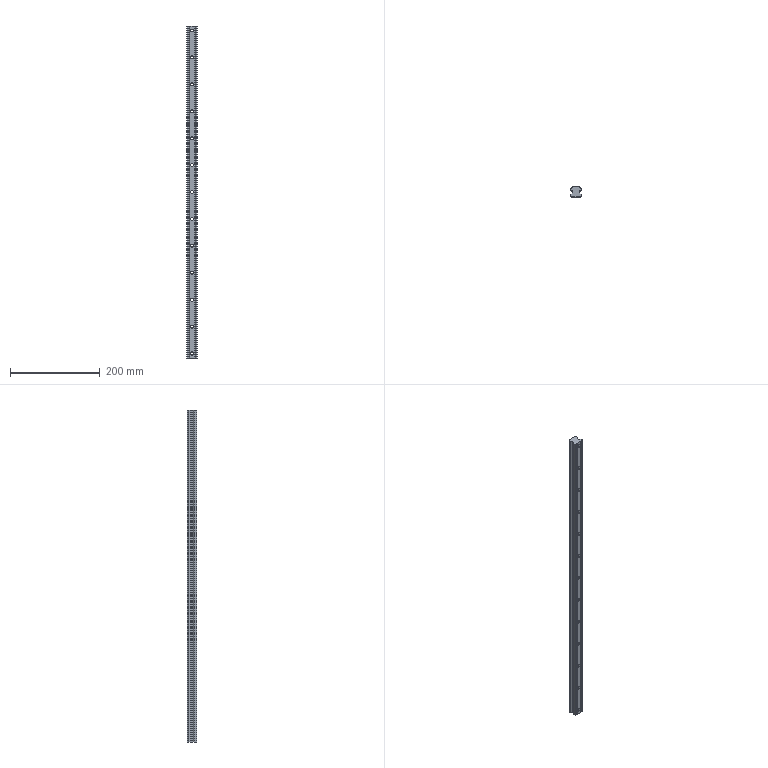Part | STEP file | HGH25 Rail | 1 solid | 99 faces | box 23 x 22 x 740 mm | volume 310065 mm3 | cylinder 56 | plane 43 | commonest cylinder face diameters 11 x26 6.6 x20 7 x6 4.6 x4